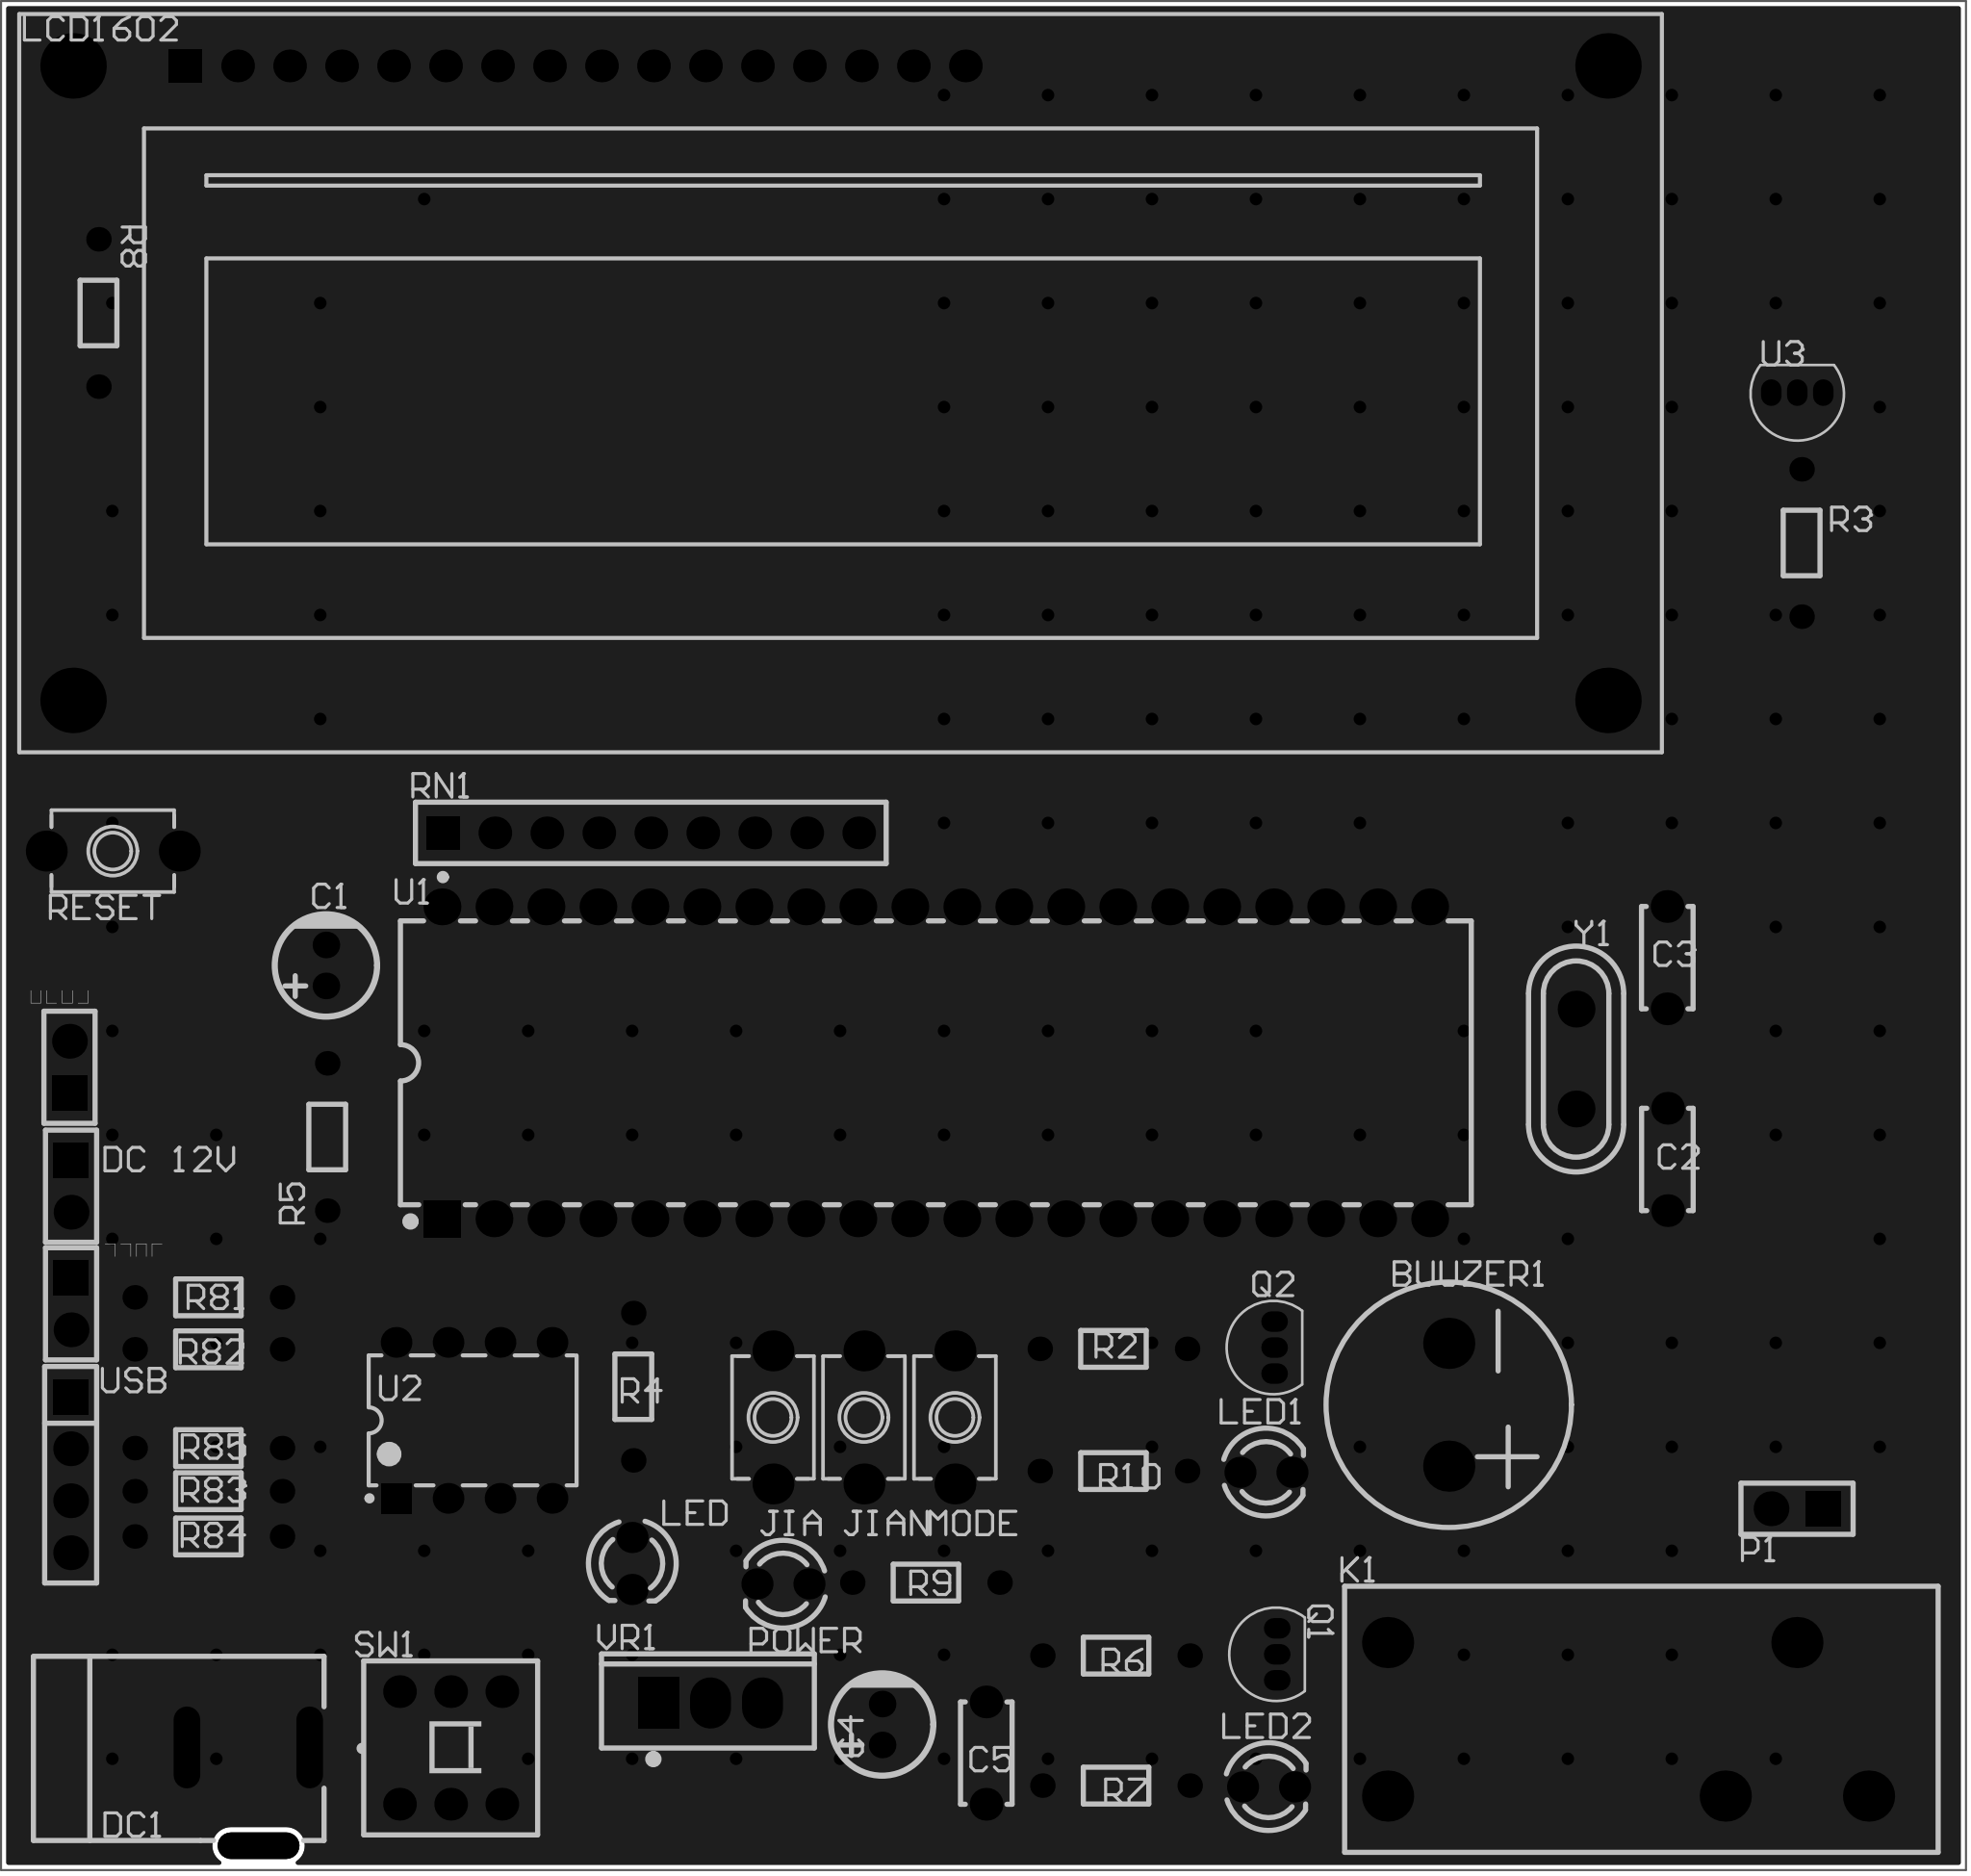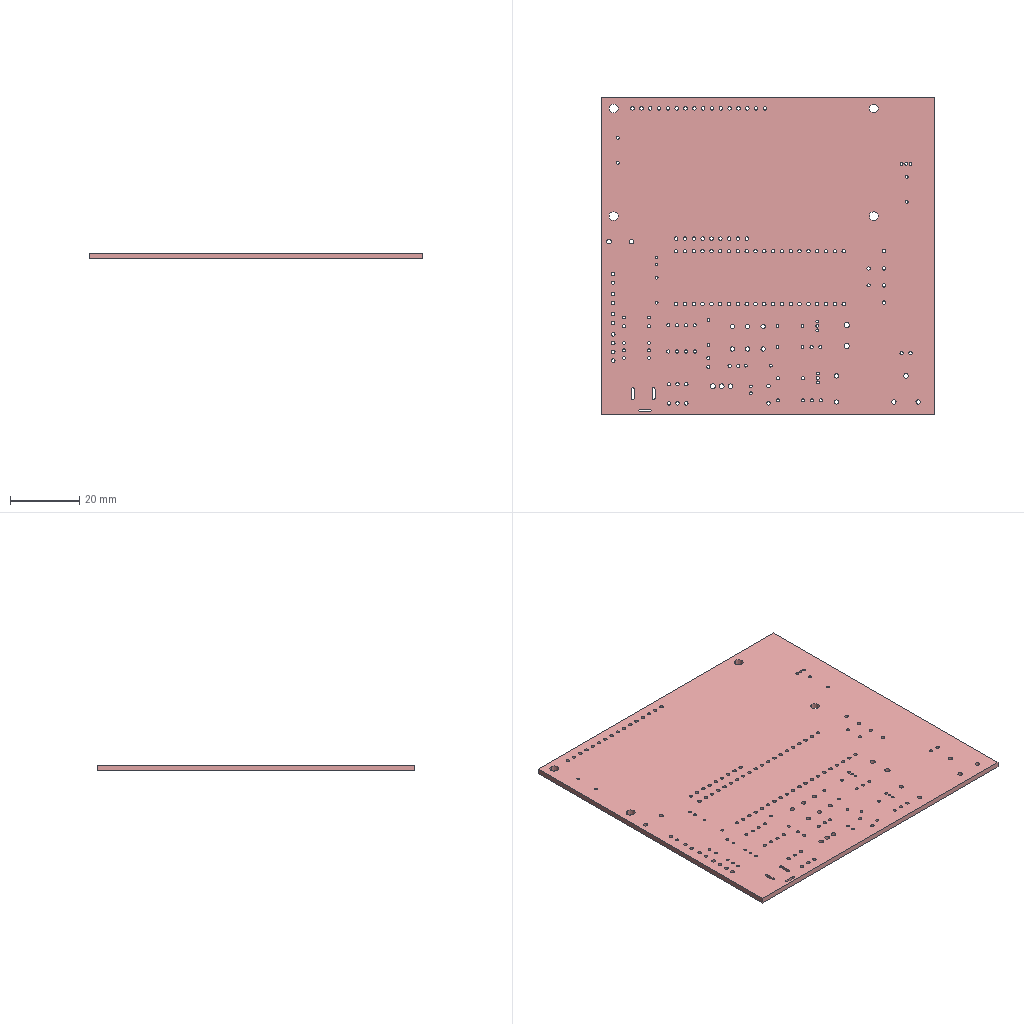Circuit board layout | Altium Designer | box 96 x 91.3 x 1.6 mm
Layer stack:
# Altium Designer layer stack of  (unit mm; dielectric type: 0 none, 1 core, 2 prepreg, 3 surface material)
index,name,kind,layer,copper_thickness_mm,dielectric_type,dielectric_thickness_mm,dielectric_material,dielectric_constant
0,Top Paste Mask Layer,other,,,,,,
1,Top Silkscreen Layer,other,,,,,,
2,Top Solder Mask Layer,dielectric,,,3,0.01,,3.3
3,Top Layer,copper,Top Layer,0.035,,,,
4,Dielectric1,dielectric,,,3,1.51,FR4,4.5
5,Bottom Layer,copper,Bottom Layer,0.035,,,,
6,Bottom Solder Mask Layer,dielectric,,,3,0.01,,3.3
7,Bottom Silkscreen Layer,other,,,,,,
8,Bottom Paste Mask Layer,other,,,,,,
# drill layer pairs: low layer,high layer
drill_pair,Top Layer,Bottom Layer
Part placement:
Designator,Comment,Layer,Footprint,Center-X(mm),Center-Y(mm),Rotation
BUUZER1,BUZZER,TopLayer,BUZ-TH_BD12.0-P6.00-D0.9-RD,153.543,107.95,270
DC1,,TopLayer,DC-2.0,94.887,88.808,180
DC 12V,Header 2,TopLayer,HDR-TH_2P-P2.54-V-F,86.225,118.628,270
JIA,SW-PB,TopLayer,KEY-TH_2P-L6.0-W3.9-P6.50,120.523,107.331,90
JIAN,SW-PB,TopLayer,KEY-TH_2P-L6.0-W3.9-P6.50,124.968,107.331,90
K1,继电器,TopLayer,RELAY-TH_G2R-1_C9900014679,162.306,92.583,0
LCD1602,LCD1602,TopLayer,LCD1602,123.825,157.861,0
LED,SI3317-H,TopLayer,LED_TH-3mm,113.635,100.195,270
LED1,SI3317-H,TopLayer,LED_TH-3mm,144.613,104.648,0
LED2,SI3317-H,TopLayer,LED_TH-3mm,144.739,89.281,0
MODE,SW-PB,TopLayer,KEY-TH_2P-L6.0-W3.9-P6.50,129.413,107.331,90
P1,Header 2,TopLayer,HDR-TH_2P-P2.54-V-F,170.561,102.87,180
POWER,SI3317-H,TopLayer,LED_TH-3mm,121.012,99.198,180
Q1,S8550,TopLayer,TO-92-3_L4.6-W3.6-P1.27-L_1,145.161,95.758,270
Q2,S8550,TopLayer,TO-92-3_L4.6-W3.6-P1.27-L_1,145.034,110.744,270
R2,470,TopLayer,Res_1/8W,137.16,110.681,180
R3,10K,TopLayer,Res_1/8W,170.785,150.053,270
R4,470,TopLayer,Res_1/8W,113.698,108.831,270
R5,10K,TopLayer,Res_1/8W,98.743,121.031,90
R6,470,TopLayer,Res_1/8W,137.287,95.695,180
R7,470,TopLayer,Res_1/8W,137.287,89.344,0
R8,470,TopLayer,Res_1/8W,87.566,161.29,270
R9,470,TopLayer,Res_1/8W,127.997,99.262,180
R10,470,TopLayer,Res_1/8W,137.16,104.711,0
R81,470,TopLayer,Res_1/8W,92.936,113.199,0
R82,470,TopLayer,Res_1/8W,92.936,110.66,180
R83,470,TopLayer,Res_1/8W,92.936,103.728,0
R84,470,TopLayer,Res_1/8W,92.936,101.516,0
R85,470,TopLayer,Res_1/8W,92.936,105.833,0
RESET,SW-PB,TopLayer,KEY-TH_2P-L6.0-W3.9-P6.50,88.265,135.001,180
RN1,-,TopLayer,RES-ARRAY-TH_9P-P2.54-D1.0,114.554,135.89,0
SW1,sw-灰色,TopLayer,SW-TH_6P-L8.5-W8.5-P2.54,104.775,91.186,0
U1,STC89C52,TopLayer,DIP-40_L52.3-W13.9-P2.54-LS15.2-BL-BASE,128.481,124.656,0
U2,ADC0832,TopLayer,DIP-8_L10.1-W6.3-P2.54-LS7.6-BL,105.918,107.188,0
U3,DS18B20,TopLayer,TO-92-3_L4.6-W3.6-P1.27-L_1,170.573,157.399,0
USB,Header 4,TopLayer,HDR-TH_4P-P2.54-V-F,86.205,104.531,270
VR1,L7805,TopLayer,TO-220AB-3_L10.4-W4.6-P2.54-L,117.472,93.38,0
Y1,11.059M,TopLayer,HC-49S_L11.0-W4.7-P4.88,159.766,124.841,270
发射线圈,Header 2,TopLayer,HDR-TH_2P-P2.54-V-F,86.148,124.439,90
接受线圈,Header 2,TopLayer,HDR-TH_2P-P2.54-V-F,86.225,112.882,270
C1,10uF,TopLayer,CAP-TH_BD5.0-P2.00-D0.8-FD-10UF50VC110GL,98.679,129.413,90
C2,18pF,TopLayer,CAP-TH_L5.0-W2.5-P5.00-D1.0,164.236,119.934,270
C3,18pF,TopLayer,CAP-TH_L5.0-W2.5-P5.00-D1.0,164.211,129.794,90
C4,470uF,TopLayer,CAP-TH_BD5.0-P2.00-D0.8-FD-10UF50VC110GL,125.857,92.329,90
C5,104,TopLayer,CAP-TH_L5.0-W2.5-P5.00-D1.0,130.937,90.932,90
Pad and via stacks:
# Altium Designer via and pad stacks of  (unit mm). Each distinct definition once, with the count of objects using it.
# via: kind,start_layer,end_layer,hole_mm,diameter_mm,mode(0 simple;1 top-mid-bottom;2 full stack),diameter_per_layer,count,example_net
# pad: kind,layer,hole_mm,hole_type(0 round;1 square;2 slot),plating,top_size,top_shape(1 round;2 rect;3 octagon;9 rounded rect),mid_size,bottom_size,mode,footprint,size_per_layer,count,example
pad,Multi-Layer,1.5,0,plated,2.5x2.5,1,2.5x2.5,2.5x2.5,0,BUZ-TH_BD12.0-P6.00-D0.9-RD,,2,BUUZER1.1
pad,Multi-Layer,0.8001,2,plated,4x1.3,1,4x1.3,4x1.3,0,DC-2.0,,3,DC1.2
pad,Multi-Layer,1,0,plated,1.7x1.7,2,1.7x1.7,1.7x1.7,0,HDR-TH_2P-P2.54-V-F,,4,DC 12V.1
pad,Multi-Layer,1,0,plated,1.7x1.7,1,1.7x1.7,1.7x1.7,0,HDR-TH_2P-P2.54-V-F,,4,DC 12V.2
pad,Multi-Layer,1.3,0,plated,2x2,1,2x2,2x2,0,KEY-TH_2P-L6.0-W3.9-P6.50,,8,JIA.1
pad,Multi-Layer,1.3,0,plated,2.5x2.5,1,2.5x2.5,2.5x2.5,0,RELAY-TH_G2R-1_C9900014679,,5,K1.1
pad,Multi-Layer,1,0,plated,1.6x1.6,1,1.6x1.6,1.6x1.6,0,LCD1602,,15,LCD1602.16
pad,Multi-Layer,1,0,plated,1.6x1.6,2,1.6x1.6,1.6x1.6,0,LCD1602,,1,LCD1602.1
pad,Multi-Layer,2.5,2,plated,3.2x3.2,1,3.2x3.2,3.2x3.2,0,LCD1602,,4,LCD1602.0
pad,Multi-Layer,0.9144,0,plated,1.524x1.524,1,1.524x1.524,1.524x1.524,0,LED_TH-3mm,,8,LED.1
pad,Multi-Layer,0.8,2,plated,1x1.3,1,1x1.3,1x1.3,0,TO-92-3_L4.6-W3.6-P1.27-L_1,,9,Q1.1
pad,Multi-Layer,0.8001,0,plated,1.199x1.199,1,1.199x1.199,1.199x1.199,0,Res_1/8W,,28,R2.1
pad,Multi-Layer,1,0,plated,1.6x1.6,2,1.6x1.6,1.6x1.6,0,RES-ARRAY-TH_9P-P2.54-D1.0,,1,RN1.1
pad,Multi-Layer,1,0,plated,1.6x1.6,1,1.6x1.6,1.6x1.6,0,RES-ARRAY-TH_9P-P2.54-D1.0,,8,RN1.2
pad,Multi-Layer,1,0,plated,1.6x1.6,1,1.6x1.6,1.6x1.6,0,SW-TH_6P-L8.5-W8.5-P2.54,,6,SW1.4
pad,Multi-Layer,1,0,plated,1.8x1.8,1,1.8x1.8,1.8x1.8,0,DIP-40_L52.3-W13.9-P2.54-LS15.2-BL-BASE,,39,U1.36
pad,Multi-Layer,1,0,plated,1.8x1.8,2,1.8x1.8,1.8x1.8,0,DIP-40_L52.3-W13.9-P2.54-LS15.2-BL-BASE,,1,U1.1
pad,Multi-Layer,0.9,0,plated,1.5x1.5,1,1.5x1.5,1.5x1.5,0,DIP-8_L10.1-W6.3-P2.54-LS7.6-BL,,7,U2.5
pad,Multi-Layer,0.9,0,plated,1.5x1.5,2,1.5x1.5,1.5x1.5,0,DIP-8_L10.1-W6.3-P2.54-LS7.6-BL,,1,U2.1
pad,Multi-Layer,1.1,0,plated,1.7x1.7,2,1.7x1.7,1.7x1.7,0,HDR-TH_4P-P2.54-V-F,,1,USB.1
pad,Multi-Layer,1.1,0,plated,1.7x1.7,1,1.7x1.7,1.7x1.7,0,HDR-TH_4P-P2.54-V-F,,3,USB.2
pad,Multi-Layer,1.4,0,plated,2x2.5,1,2x2.5,2x2.5,0,TO-220AB-3_L10.4-W4.6-P2.54-L,,2,VR1.2
pad,Multi-Layer,1.4,0,plated,2x2.5,2,2x2.5,2x2.5,0,TO-220AB-3_L10.4-W4.6-P2.54-L,,1,VR1.1
pad,Multi-Layer,0.9,0,plated,1.8x1.8,1,1.8x1.8,1.8x1.8,0,HC-49S_L11.0-W4.7-P4.88,,2,Y1.1
pad,Multi-Layer,0.8,0,plated,1.3x1.3,1,1.3x1.3,1.3x1.3,0,CAP-TH_BD5.0-P2.00-D0.8-FD-10UF50VC110GL,,4,C1.2
pad,Multi-Layer,1,0,plated,1.6x1.6,1,1.6x1.6,1.6x1.6,0,CAP-TH_L5.0-W2.5-P5.00-D1.0,,6,C2.1
via,Top Layer,Bottom Layer,0.3048,0.61,0,,182,GND
Copper pours:
name,layer,net,type(0 solid;1 hatched;2 none)
Bottom Layer-GND,Bottom Layer,GND,0
Top Layer-GND,Top Layer,GND,0
Design rules, without the lines most boards share:
# Altium Designer design rules of  (exported by Altium Designer, unit mm)
# columns: name | kind | enabled | priority | scope1 | scope2 | descriptor | typed fields (field=value)
creepage | 65 | enabled | 1 | All | All | Creepage Distance Constraint =(0mil) (All),(All) |